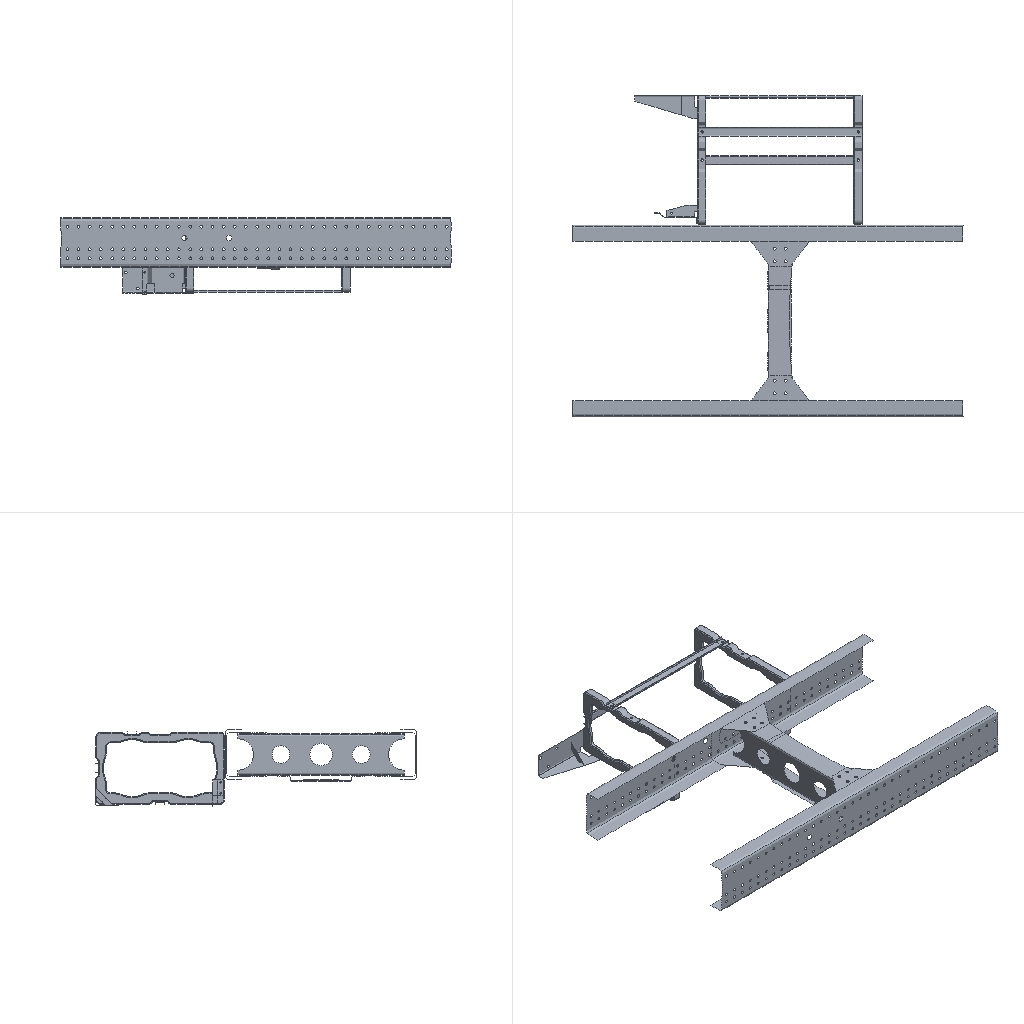Simulation study | nastran
Set-up summary:
category,name,step,type,value,unit,region
solver,nx_nastran
units,not stated in the deck,,not stated
analysis,deck,,static,static
analysis,solution,,SOL,101
load_step,SUBCASE 1,1,SUBCASE,SPC=6 LOAD=1
load_step,SUBCASE 2,2,SUBCASE,SPC=6 LOAD=2
load_step,SUBCASE 3,3,SUBCASE,SPC=6 LOAD=3
load_step,SUBCASE 4,4,SUBCASE,SPC=6 LOAD=4
load_step,requested,,,4
mesh,nodes,,,42307
mesh,elements,,,39229
element_type,CONM2,,mass,2
element_type,CQUAD4,,shell,38735
element_type,CTRIA3,,shell,492
load,load commands in deck,,count,4
bc,support commands in deck,,count,146
check,setup vs results,,match,"every grid point's frame and coordinates and every element id; grid points of CQUAD4, CTRIA3 elements"
Nastran input file, long lists of numbers shortened:
$$------------------------------------------------------------------------------$
$$                                                                              $
$$ NASTRAN Input Deck Generated by HyperMesh Version  : 9.0b121                 $
$$ Generated using HyperMesh-Nastran Template Version : 9.0b121
$$                                                                              $
$$   Template:  general                                                         $
$$                                                                              $
$$------------------------------------------------------------------------------$
$$------------------------------------------------------------------------------$
$$                      Executive Control Cards                                 $
$$------------------------------------------------------------------------------$
SOL 101
CEND
$$------------------------------------------------------------------------------$
$$                      Case Control Cards                                      $
$$------------------------------------------------------------------------------$
  DISPLACEMENT(PLOT) = ALL
  STRESS(PLOT) = ALL
  STRAIN(PLOT) = ALL
$
$HMNAME LOADSTEP               1"Step_X2g"
SUBCASE       1
  LABEL=     Step_X2g
  SPC =        6
  LOAD =        1
$
$HMNAME LOADSTEP               2"Step_Y2g"
SUBCASE       2
  LABEL=     Step_Y2g
  SPC =        6
  LOAD =        2
$
$HMNAME LOADSTEP               3"Step_Z2g"
SUBCASE       3
  LABEL=     Step_Z2g
  SPC =        6
  LOAD =        3
$
$HMNAME LOADSTEP               4"Step_Z-4g"
SUBCASE       4
  LABEL=     Step_Z-4g
  SPC =        6
  LOAD =        4
$$------------------------------------------------------------------------------$
$$                      Bulk Data Cards                                         $
$$------------------------------------------------------------------------------$
BEGIN BULK
PARAM,BAILOUT,-1
PARAM,POST,-1
$$
$$  GRID Data
$$
GRID         221        2250.0  962.2293-337.5
GRID         222        2254.623963.5064-337.5
$ (42305 more lines like these left out)
$$
$$  SPOINT Data
$$
$
$  CONM2 Elements
$
CONM2     185904  219877       00.0046  0.0     0.0     0.0
CONM2     185905  219712       00.016   0.0     0.0     0.0
$
$HMMOVE        8
$         185904THRU      185905
$
$$
$$------------------------------------------------------------------------------$
$$             Group Definitions                                                $
$$------------------------------------------------------------------------------$
$$
$$ RBE2 Elements - Multiple dependent nodes
$$
RBE2      185762  219712   12346    4052    4053    4054    4055    4056+
+           4057    4058    4059    4060    4061    4062    4063    4064+
+           4071    4072    4073    4074    4075    4076    4077    4078+
+           4079    4080    4081    4082    4083    4084    4092    4093+
+           4094    4095    4096    4097    4098    4099    4100    4102+
+           4103    4104    4497    4498    4499    4500    4501    4502+
+           4503    4504    4505    4506    4507    4508    4509    4524+
+           4525    4526    4527    4528    4529    4530    4531    4532+
+           4533    4534    4535    4536    4537    4550    4551    4552+
+           4553    4554    4555    4556    4557    4558    4559    4560+
+           4561    4754    4755    4756    4757    4758    4759    4760+
+           4761    4762    4763    4764    4765    4766    4767    4768+
+           4769    4794    4795    4796    4797    4798    4799    4800+
+           4801    4802  205453  205454  205455  205456  205457  205458+
+         205459  205460  205461  205462  205463  205464  205465  205466+
+         205467  205468  205469    5199    5200    5201    5202    5203+
+           5204    5205    5206    5207    5208    5209    5210    5211+
+           5224    5225    5226    5227    5228    5229    5230    5231+
+           5232    5233    5234    5235    5236    5237    5238    5239+
+           5240    5241    5242    5243    5244    5245    5246    5248+
+           5249    5250  205535  205536  205546  205547    6167    6182+
+         205620  205621  205622  205623  205624  205625  205626  205627+
+         205628  205629  205630  205631  205632  205633  205634  205635+
+         205636  205637  205638  205639  205640  205641  205642  205643+
+         205644  205645  205646  205647  205648  205649  205790  205791+
+         205792  205793  205794  205795  205796  205797  205798  205799+
+         205800  205832  205833  205834  205835  205836  205837  205838+
+         205839  205840  205841  205842  205844  205845  205846  205847+
+         205848  205849  205850  205851  205852  205853  205854  206515+
+         206516  206517  206518  206519  206520  206521  206522  206523+
+         206524  206525  206526  206527  206528  206529  206530  206531+
+         206532  206533  206534  206535  206536  206548  206549  206550+
+         206551  206552  206553  206554  206555  206556  206557    7983+
+         206558  206559  206560  206561  206562  206563  206564  206565+
+         206566  206567  206568  206574  206575  206583  206584  206585+
+         206586  206587  206588  206589  206590  206591  206592  206593+
+         206594  206595  206596  206597  206598  206599  206600  206601+
+         206603  207196  207201  207202  207204  207205  207206  207207+
+         207208  207209  207210  207214  207216  207219  207220  207265+
+         207266  207267  207268  207269    9101  207276  207293  207294+
+         207295  207303  207306  207318  207319  207320  207323  207324+
+         209700  209703  209704  209708  209713  209715  209717  209718+
+         209719  209750  209751  209754  209757  209758  209759  209760+
+         209766  209769  209770  209772  209776   12137   12138   12139+
+          12140   12142  209778   12148  209783  209784  209785   12161+
+          12163  209828  209830  209831  209832  209833  209834  209837+
+         209838  209839  209841  209842  209843  209844   12231   12233+
+          12238   12239   12240   12241   12242   12243   12244   12245+
+         209845  209846  209850  209851  209852  209853  209854  210174+
+         210175  210176  210177  210178  210179  210180  210181  210182+
+         210183  210184  210185  210186  210187  210188  210189  210190+
+         210191  210192  210193  210194  210195  210196  210197  210198+
+         210199  210579  210580  210581  210582  210583  210584  210585+
+         210586  210587  210588  210589  210590  210591  210604  210605+
+         210606  210607  210608  210609  210610  210611  210612  210613+
+         210614  210615  210616  210617  210618  210619  210620  210621+
+         210622  210623  210624  210625  210626  210628  210629  210630+
+         210839  210954   13435  210955  210956  210957  210958  210959+
+         210960  210961  210962  210963  210964   13446   13447  210965+
+          13449  210966  210967  210968  210969  210970  210971  211003+
+         211004  211010  211013  211014  211015   13535  211017  211032+
+          13555   13556  211039   13565  211285  211286  211287  211288+
+         211289  211290  211291  211292  211293  211294  211295  211327+
+         211328  211329  211330  211331  211332  211333  211334  211335+
+         211336  211337  211339  211340  211341  211342  211343  211344+
+         211345  211346  211347  211348  211349  212069  212070  212071+
+         212072  212073  212074  212075  212076  212077  212078  212079+
+         212080  212081  212082  212083  212084  212085  212086  212087+
+         212088  212089  212090  212102  212103  212104  212105  212106+
+         212107  212108  212109  212110  212111  212112  212113  212114+
+         212115  212116  212117  212118  212119  212120  212121  212122+
+         212123  212129  212130  212138  212139  212140  212141  212142+
+         212143  212144  212145  212146  212147  212148  212149  212150+
+         212151  212152  212153  212154  212155  212156  212158
RBE2      185763  219713   12346    3188    3189    3190    3191    3192+
+           3193    3194    3195    3196    3197    3198    3199    3200+
+           3201    3202    3203  219631  219632  219633  219639  219640+
+         219642  219643  219650
$ (306 more lines like these left out)
$
$HMMOVE        7
$         185762THRU      185774  185903  813136THRU      813139  813141THRU
$         813158  813166THRU      813174  813176THRU      813188
$
$$
$$  CTRIA3 Data
$$
CTRIA3       113       7     373     374  203902
CTRIA3      3265       7    4030    4029    4025
$ (490 more lines like these left out)
$
$HMMOVE        3
$            113    3265    3574    3595    3599    3604    3613    3623    3625
$       THRU        3626    3772    3805    3926    4144    4203    4230    4234
$ (81 more lines like these left out)
CQUAD4        74       7     289     302     291     288
CQUAD4        76       7     290     301     302     289
$ (38733 more lines like these left out)
$
$HMMOVE        3
$             74      76THRU          88     114THRU         115     133THRU
$            134     184THRU         216     218     220THRU         234     236
$ (830 more lines like these left out)
PSHELL         7      353.0           35              35
$
$HMNAME PROP                   9"Sheel_500T" 4
$HWCOLOR PROP                  9       5
PSHELL         9      355.0           35              35
$
$HMNAME PROP                  12"Sheel_600T" 4
$HWCOLOR PROP                 12       3
PSHELL        12      356.0           35              35
$
$HMNAME PROP                  13"Sheel_400T" 4
$HWCOLOR PROP                 13       3
PSHELL        13      354.0           35              35
$$
$$------------------------------------------------------------------------------$
$$                      Material Definition Cards                               $
$$------------------------------------------------------------------------------$
$$--------------------------------------------------------------
$$ HYPERMESH TAGS
$$--------------------------------------------------------------
$$BEGIN TAGS
$$END TAGS
$$
$$  MAT1 Data
$
$HMNAME MAT                   35"steel" "MAT1"
$HWCOLOR MAT                  35       6
MAT1          35210000.0        0.3     7.80E-09
$$
$$
$$
$$------------------------------------------------------------------------------$
$ (27 more lines like these left out)
GRAV           1        9800.0  2.0     0.0     0.0
$$
$HMNAME LOADCOL                2"Y2g"
$HWCOLOR LOADCOL               2       4
GRAV           2        9800.0  0.0     2.0     0.0
$$
$HMNAME LOADCOL                3"Z2g"
$HWCOLOR LOADCOL               3       5
GRAV           3        9800.0  0.0     0.0     2.0
$$
$HMNAME LOADCOL                4"Z-4g"
$HWCOLOR LOADCOL               4       6
GRAV           4        9800.0  0.0     0.0     -4.0
$$
$$
$$
$$
$$
$$
$$
$$
$$
$$
$$
$$  SPC Data
$$
SPC            6  107038  12346 0.0
SPC            6  107036  12346 0.0
SPC            6  105802  12346 0.0
SPC            6  105800  12346 0.0
$ (142 more lines like these left out)
$HMASSEM   28010       3 2801
$HMASSEM_IDS     2801005 2801007 2801015 2801014
$
ENDDATA
Results summary:
result,analysis,,,static
result,last_loadstep,,,4
result,primary field,,,displacements
result,max displacement,,,1.637,model units